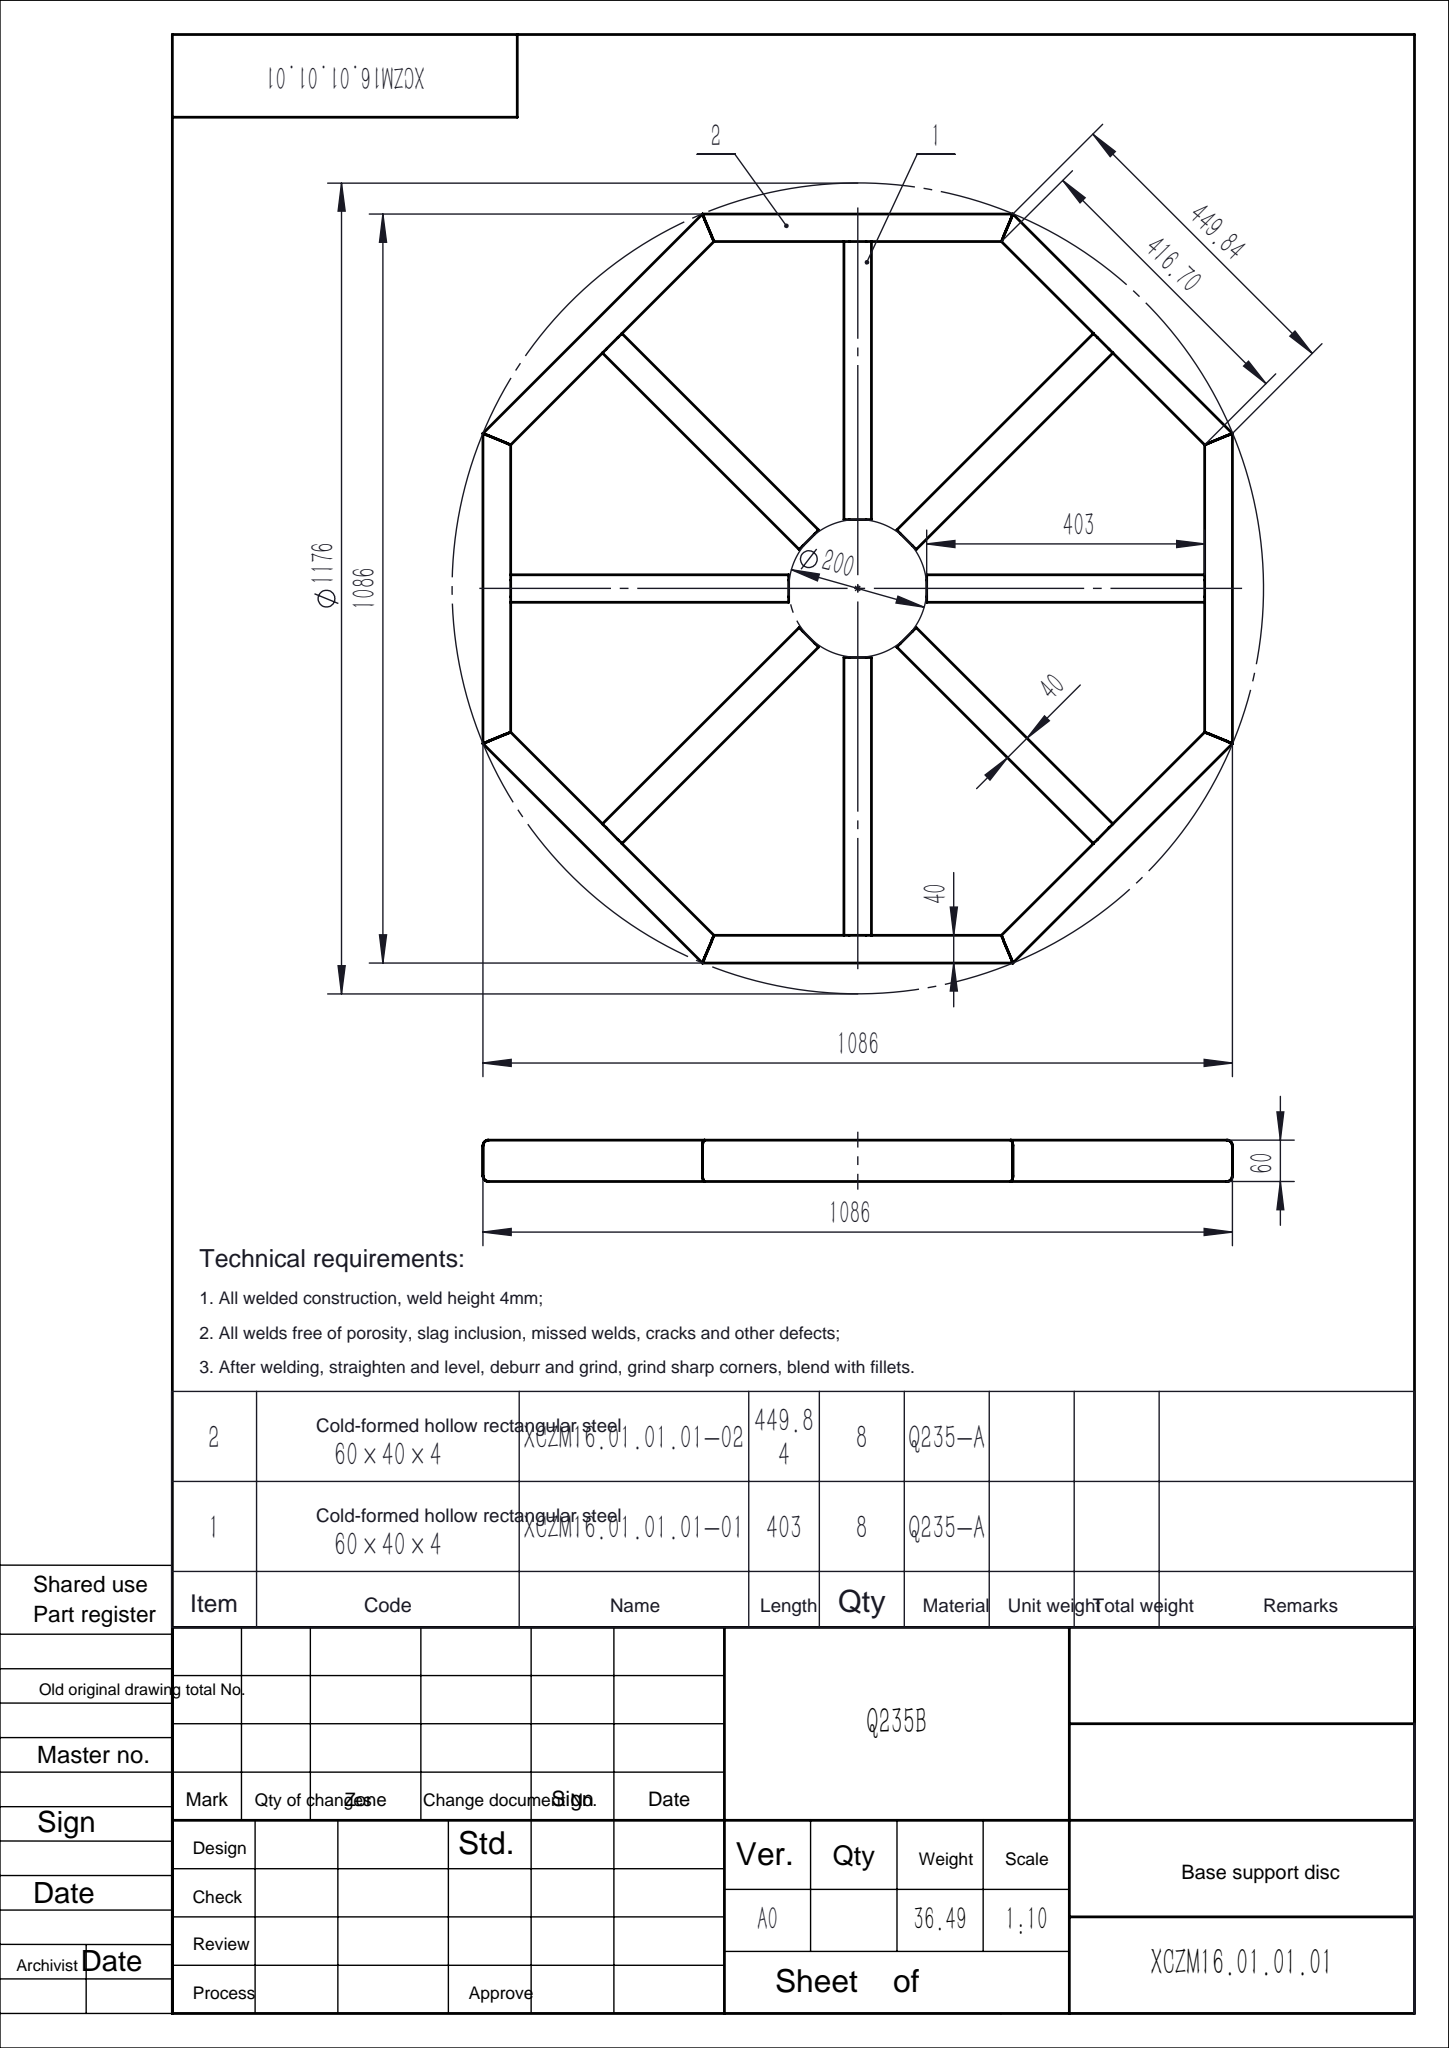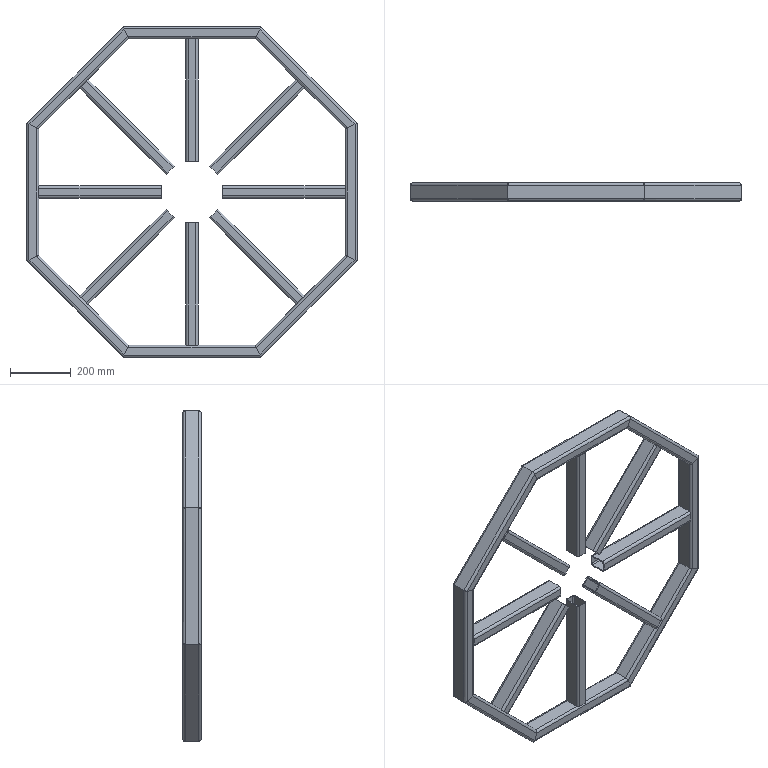Part | SolidWorks | features WeldCornerFeat 8, CirPattern 1, RefAxis 1, WeldMemberFeat 1, WeldmentFeature 1 | 16 solids | 288 faces | box 1086 x 60 x 1086 mm | volume 4648285 mm3 | plane 160 | cylinder 128 | commonest cylinder face diameters 8 x64 16 x64